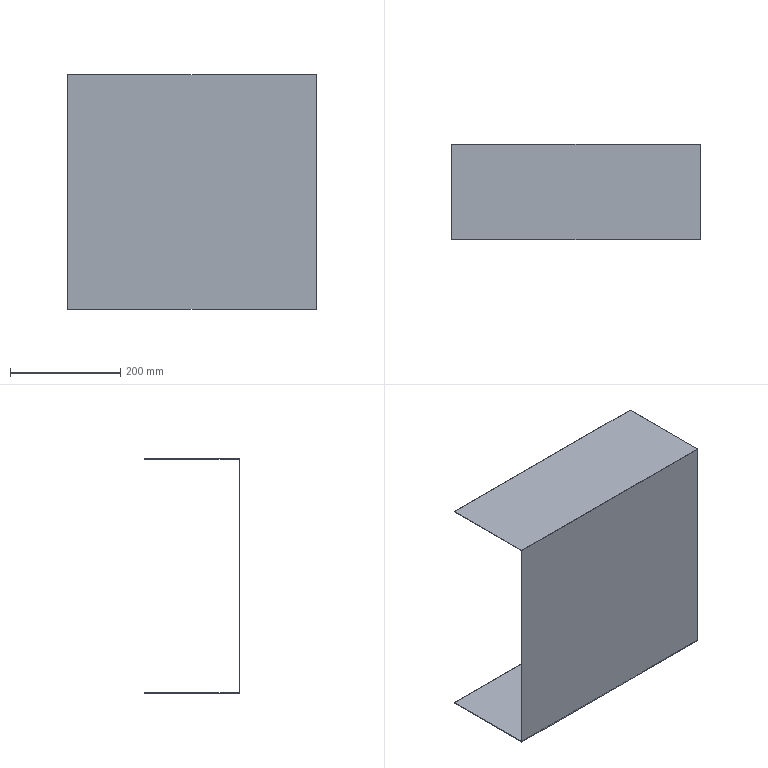Part | STEP file | Chassis side seal plate B_RR | 1 solid | 10 faces | box 450 x 173 x 425 mm | volume 346050 mm3 | plane 10
STEP:
#1=CARTESIAN_POINT('',(0.,0.,0.));
#2=DIRECTION('',(0.,0.,1.));
#3=DIRECTION('',(1.,0.,0.));
#4=AXIS2_PLACEMENT_3D('',#1,#2,#3);
#5=CARTESIAN_POINT('',(225.,0.,212.5));
#6=VERTEX_POINT('',#5);
#7=CARTESIAN_POINT('',(225.,0.,-212.5));
#8=VERTEX_POINT('',#7);
#9=CARTESIAN_POINT('',(225.,0.,0.));
#10=DIRECTION('',(0.,0.,-1.));
#11=VECTOR('',#10,1.);
#12=LINE('',#9,#11);
#13=CARTESIAN_POINT('',(0.,0.,0.));
#14=DIRECTION('',(0.,1.,0.));
#15=DIRECTION('',(0.,0.,1.));
#16=AXIS2_PLACEMENT_3D('',#13,#14,#15);
#17=PLANE('',#16);
#18=CARTESIAN_POINT('',(0.,225.));
#19=DIRECTION('',(-1.,0.));
#20=VECTOR('',#19,1.);
#21=LINE('',#18,#20);
#22=(GEOMETRIC_REPRESENTATION_CONTEXT(2)PARAMETRIC_REPRESENTATION_CONTEXT()REPRESENTATION_CONTEXT('',''));
#23=DEFINITIONAL_REPRESENTATION('',(#21),#22);
#24=PCURVE('',#17,#23);
#25=CARTESIAN_POINT('',(225.,0.,212.5));
#26=DIRECTION('',(1.,0.,0.));
#27=DIRECTION('',(0.,0.,-1.));
#28=AXIS2_PLACEMENT_3D('',#25,#26,#27);
#29=PLANE('',#28);
#30=CARTESIAN_POINT('',(212.5,0.));
#31=DIRECTION('',(1.,0.));
#32=VECTOR('',#31,1.);
#33=LINE('',#30,#32);
#34=(GEOMETRIC_REPRESENTATION_CONTEXT(2)PARAMETRIC_REPRESENTATION_CONTEXT()REPRESENTATION_CONTEXT('',''));
#35=DEFINITIONAL_REPRESENTATION('',(#33),#34);
#36=PCURVE('',#29,#35);
#37=SURFACE_CURVE('',#12,(#24,#36),.PCURVE_S1.);
#38=EDGE_CURVE('',#6,#8,#37,.T.);
#39=ORIENTED_EDGE('',*,*,#38,.F.);
#40=CARTESIAN_POINT('',(-225.,0.,212.5));
#41=VERTEX_POINT('',#40);
#42=CARTESIAN_POINT('',(0.,0.,212.5));
#43=DIRECTION('',(1.,0.,0.));
#44=VECTOR('',#43,1.);
#45=LINE('',#42,#44);
#46=CARTESIAN_POINT('',(212.5,0.));
#47=DIRECTION('',(0.,1.));
#48=VECTOR('',#47,1.);
#49=LINE('',#46,#48);
#50=(GEOMETRIC_REPRESENTATION_CONTEXT(2)PARAMETRIC_REPRESENTATION_CONTEXT()REPRESENTATION_CONTEXT('',''));
#51=DEFINITIONAL_REPRESENTATION('',(#49),#50);
#52=PCURVE('',#17,#51);
#53=CARTESIAN_POINT('',(-225.,0.,212.5));
#54=DIRECTION('',(0.,0.,1.));
#55=DIRECTION('',(1.,0.,0.));
#56=AXIS2_PLACEMENT_3D('',#53,#54,#55);
#57=PLANE('',#56);
#58=CARTESIAN_POINT('',(225.,0.));
#59=DIRECTION('',(1.,0.));
#60=VECTOR('',#59,1.);
#61=LINE('',#58,#60);
#62=(GEOMETRIC_REPRESENTATION_CONTEXT(2)PARAMETRIC_REPRESENTATION_CONTEXT()REPRESENTATION_CONTEXT('',''));
#63=DEFINITIONAL_REPRESENTATION('',(#61),#62);
#64=PCURVE('',#57,#63);
#65=SURFACE_CURVE('',#45,(#52,#64),.PCURVE_S1.);
#66=EDGE_CURVE('',#41,#6,#65,.T.);
#67=ORIENTED_EDGE('',*,*,#66,.F.);
#68=CARTESIAN_POINT('',(-225.,0.,-212.5));
#69=VERTEX_POINT('',#68);
#70=CARTESIAN_POINT('',(-225.,0.,0.));
#71=DIRECTION('',(0.,0.,1.));
#72=VECTOR('',#71,1.);
#73=LINE('',#70,#72);
#74=CARTESIAN_POINT('',(0.,-225.));
#75=DIRECTION('',(1.,0.));
#76=VECTOR('',#75,1.);
#77=LINE('',#74,#76);
#78=(GEOMETRIC_REPRESENTATION_CONTEXT(2)PARAMETRIC_REPRESENTATION_CONTEXT()REPRESENTATION_CONTEXT('',''));
#79=DEFINITIONAL_REPRESENTATION('',(#77),#78);
#80=PCURVE('',#17,#79);
#81=CARTESIAN_POINT('',(-225.,0.,-212.5));
#82=DIRECTION('',(-1.,0.,0.));
#83=DIRECTION('',(0.,0.,1.));
#84=AXIS2_PLACEMENT_3D('',#81,#82,#83);
#85=PLANE('',#84);
#86=CARTESIAN_POINT('',(212.5,0.));
#87=DIRECTION('',(1.,0.));
#88=VECTOR('',#87,1.);
#89=LINE('',#86,#88);
#90=(GEOMETRIC_REPRESENTATION_CONTEXT(2)PARAMETRIC_REPRESENTATION_CONTEXT()REPRESENTATION_CONTEXT('',''));
#91=DEFINITIONAL_REPRESENTATION('',(#89),#90);
#92=PCURVE('',#85,#91);
#93=SURFACE_CURVE('',#73,(#80,#92),.PCURVE_S1.);
#94=EDGE_CURVE('',#69,#41,#93,.T.);
#95=ORIENTED_EDGE('',*,*,#94,.F.);
#96=CARTESIAN_POINT('',(0.,0.,-212.5));
#97=DIRECTION('',(-1.,0.,0.));
#98=VECTOR('',#97,1.);
#99=LINE('',#96,#98);
#100=CARTESIAN_POINT('',(-212.5,0.));
#101=DIRECTION('',(0.,-1.));
#102=VECTOR('',#101,1.);
#103=LINE('',#100,#102);
#104=(GEOMETRIC_REPRESENTATION_CONTEXT(2)PARAMETRIC_REPRESENTATION_CONTEXT()REPRESENTATION_CONTEXT('',''));
#105=DEFINITIONAL_REPRESENTATION('',(#103),#104);
#106=PCURVE('',#17,#105);
#107=CARTESIAN_POINT('',(225.,0.,-212.5));
#108=DIRECTION('',(0.,0.,-1.));
#109=DIRECTION('',(-1.,0.,0.));
#110=AXIS2_PLACEMENT_3D('',#107,#108,#109);
#111=PLANE('',#110);
#112=CARTESIAN_POINT('',(225.,0.));
#113=DIRECTION('',(1.,0.));
#114=VECTOR('',#113,1.);
#115=LINE('',#112,#114);
#116=(GEOMETRIC_REPRESENTATION_CONTEXT(2)PARAMETRIC_REPRESENTATION_CONTEXT()REPRESENTATION_CONTEXT('',''));
#117=DEFINITIONAL_REPRESENTATION('',(#115),#116);
#118=PCURVE('',#111,#117);
#119=SURFACE_CURVE('',#99,(#106,#118),.PCURVE_S1.);
#120=EDGE_CURVE('',#8,#69,#119,.T.);
#121=ORIENTED_EDGE('',*,*,#120,.F.);
#122=EDGE_LOOP('',(#39,#67,#95,#121));
#123=FACE_BOUND('',#122,.T.);
#124=ADVANCED_FACE('',(#123),#17,.F.);
#125=CARTESIAN_POINT('',(225.,173.,-212.5));
#126=VERTEX_POINT('',#125);
#127=CARTESIAN_POINT('',(225.,0.,-212.5));
#128=DIRECTION('',(0.,-1.,0.));
#129=VECTOR('',#128,1.);
#130=LINE('',#127,#129);
#131=CARTESIAN_POINT('',(0.,0.));
#132=DIRECTION('',(0.,-1.));
#133=VECTOR('',#132,1.);
#134=LINE('',#131,#133);
#135=(GEOMETRIC_REPRESENTATION_CONTEXT(2)PARAMETRIC_REPRESENTATION_CONTEXT()REPRESENTATION_CONTEXT('',''));
#136=DEFINITIONAL_REPRESENTATION('',(#134),#135);
#137=PCURVE('',#111,#136);
#138=CARTESIAN_POINT('',(425.,0.));
#139=DIRECTION('',(0.,-1.));
#140=VECTOR('',#139,1.);
#141=LINE('',#138,#140);
#142=(GEOMETRIC_REPRESENTATION_CONTEXT(2)PARAMETRIC_REPRESENTATION_CONTEXT()REPRESENTATION_CONTEXT('',''));
#143=DEFINITIONAL_REPRESENTATION('',(#141),#142);
#144=PCURVE('',#29,#143);
#145=SURFACE_CURVE('',#130,(#137,#144),.PCURVE_S1.);
#146=EDGE_CURVE('',#126,#8,#145,.T.);
#147=ORIENTED_EDGE('',*,*,#146,.T.);
#148=ORIENTED_EDGE('',*,*,#120,.T.);
#149=CARTESIAN_POINT('',(-225.,173.,-212.5));
#150=VERTEX_POINT('',#149);
#151=CARTESIAN_POINT('',(-225.,0.,-212.5));
#152=DIRECTION('',(0.,1.,0.));
#153=VECTOR('',#152,1.);
#154=LINE('',#151,#153);
#155=CARTESIAN_POINT('',(450.,0.));
#156=DIRECTION('',(0.,1.));
#157=VECTOR('',#156,1.);
#158=LINE('',#155,#157);
#159=(GEOMETRIC_REPRESENTATION_CONTEXT(2)PARAMETRIC_REPRESENTATION_CONTEXT()REPRESENTATION_CONTEXT('',''));
#160=DEFINITIONAL_REPRESENTATION('',(#158),#159);
#161=PCURVE('',#111,#160);
#162=CARTESIAN_POINT('',(0.,0.));
#163=DIRECTION('',(0.,1.));
#164=VECTOR('',#163,1.);
#165=LINE('',#162,#164);
#166=(GEOMETRIC_REPRESENTATION_CONTEXT(2)PARAMETRIC_REPRESENTATION_CONTEXT()REPRESENTATION_CONTEXT('',''));
#167=DEFINITIONAL_REPRESENTATION('',(#165),#166);
#168=PCURVE('',#85,#167);
#169=SURFACE_CURVE('',#154,(#161,#168),.PCURVE_S1.);
#170=EDGE_CURVE('',#69,#150,#169,.T.);
#171=ORIENTED_EDGE('',*,*,#170,.T.);
#172=CARTESIAN_POINT('',(225.,173.,-212.5));
#173=DIRECTION('',(1.,0.,0.));
#174=VECTOR('',#173,1.);
#175=LINE('',#172,#174);
#176=CARTESIAN_POINT('',(0.,173.));
#177=DIRECTION('',(-1.,0.));
#178=VECTOR('',#177,1.);
#179=LINE('',#176,#178);
#180=(GEOMETRIC_REPRESENTATION_CONTEXT(2)PARAMETRIC_REPRESENTATION_CONTEXT()REPRESENTATION_CONTEXT('',''));
#181=DEFINITIONAL_REPRESENTATION('',(#179),#180);
#182=PCURVE('',#111,#181);
#183=CARTESIAN_POINT('',(0.,173.,0.));
#184=DIRECTION('',(0.,1.,0.));
#185=DIRECTION('',(0.,0.,1.));
#186=AXIS2_PLACEMENT_3D('',#183,#184,#185);
#187=PLANE('',#186);
#188=CARTESIAN_POINT('',(-212.5,225.));
#189=DIRECTION('',(0.,1.));
#190=VECTOR('',#189,1.);
#191=LINE('',#188,#190);
#192=(GEOMETRIC_REPRESENTATION_CONTEXT(2)PARAMETRIC_REPRESENTATION_CONTEXT()REPRESENTATION_CONTEXT('',''));
#193=DEFINITIONAL_REPRESENTATION('',(#191),#192);
#194=PCURVE('',#187,#193);
#195=SURFACE_CURVE('',#175,(#182,#194),.PCURVE_S1.);
#196=EDGE_CURVE('',#150,#126,#195,.T.);
#197=ORIENTED_EDGE('',*,*,#196,.T.);
#198=EDGE_LOOP('',(#147,#148,#171,#197));
#199=FACE_BOUND('',#198,.T.);
#200=ADVANCED_FACE('',(#199),#111,.T.);
#201=CARTESIAN_POINT('',(225.,173.,-211.5));
#202=VERTEX_POINT('',#201);
#203=CARTESIAN_POINT('',(225.,1.,-211.5));
#204=VERTEX_POINT('',#203);
#205=CARTESIAN_POINT('',(225.,0.,-211.5));
#206=DIRECTION('',(0.,-1.,0.));
#207=VECTOR('',#206,1.);
#208=LINE('',#205,#207);
#209=CARTESIAN_POINT('',(424.,0.));
#210=DIRECTION('',(0.,-1.));
#211=VECTOR('',#210,1.);
#212=LINE('',#209,#211);
#213=(GEOMETRIC_REPRESENTATION_CONTEXT(2)PARAMETRIC_REPRESENTATION_CONTEXT()REPRESENTATION_CONTEXT('',''));
#214=DEFINITIONAL_REPRESENTATION('',(#212),#213);
#215=PCURVE('',#29,#214);
#216=CARTESIAN_POINT('',(225.,0.,-211.5));
#217=DIRECTION('',(0.,0.,-1.));
#218=DIRECTION('',(-1.,0.,0.));
#219=AXIS2_PLACEMENT_3D('',#216,#217,#218);
#220=PLANE('',#219);
#221=CARTESIAN_POINT('',(0.,0.));
#222=DIRECTION('',(0.,-1.));
#223=VECTOR('',#222,1.);
#224=LINE('',#221,#223);
#225=(GEOMETRIC_REPRESENTATION_CONTEXT(2)PARAMETRIC_REPRESENTATION_CONTEXT()REPRESENTATION_CONTEXT('',''));
#226=DEFINITIONAL_REPRESENTATION('',(#224),#225);
#227=PCURVE('',#220,#226);
#228=SURFACE_CURVE('',#208,(#215,#227),.PCURVE_S1.);
#229=EDGE_CURVE('',#202,#204,#228,.T.);
#230=ORIENTED_EDGE('',*,*,#229,.T.);
#231=CARTESIAN_POINT('',(225.,1.,211.5));
#232=VERTEX_POINT('',#231);
#233=CARTESIAN_POINT('',(225.,1.,212.5));
#234=DIRECTION('',(0.,0.,1.));
#235=VECTOR('',#234,1.);
#236=LINE('',#233,#235);
#237=CARTESIAN_POINT('',(0.,1.));
#238=DIRECTION('',(-1.,0.));
#239=VECTOR('',#238,1.);
#240=LINE('',#237,#239);
#241=(GEOMETRIC_REPRESENTATION_CONTEXT(2)PARAMETRIC_REPRESENTATION_CONTEXT()REPRESENTATION_CONTEXT('',''));
#242=DEFINITIONAL_REPRESENTATION('',(#240),#241);
#243=PCURVE('',#29,#242);
#244=CARTESIAN_POINT('',(0.,1.,0.));
#245=DIRECTION('',(0.,1.,0.));
#246=DIRECTION('',(0.,0.,1.));
#247=AXIS2_PLACEMENT_3D('',#244,#245,#246);
#248=PLANE('',#247);
#249=CARTESIAN_POINT('',(212.5,225.));
#250=DIRECTION('',(1.,0.));
#251=VECTOR('',#250,1.);
#252=LINE('',#249,#251);
#253=(GEOMETRIC_REPRESENTATION_CONTEXT(2)PARAMETRIC_REPRESENTATION_CONTEXT()REPRESENTATION_CONTEXT('',''));
#254=DEFINITIONAL_REPRESENTATION('',(#252),#253);
#255=PCURVE('',#248,#254);
#256=SURFACE_CURVE('',#236,(#243,#255),.PCURVE_S1.);
#257=EDGE_CURVE('',#204,#232,#256,.T.);
#258=ORIENTED_EDGE('',*,*,#257,.T.);
#259=CARTESIAN_POINT('',(225.,173.,211.5));
#260=VERTEX_POINT('',#259);
#261=CARTESIAN_POINT('',(225.,0.,211.5));
#262=DIRECTION('',(0.,1.,0.));
#263=VECTOR('',#262,1.);
#264=LINE('',#261,#263);
#265=CARTESIAN_POINT('',(1.,0.));
#266=DIRECTION('',(0.,1.));
#267=VECTOR('',#266,1.);
#268=LINE('',#265,#267);
#269=(GEOMETRIC_REPRESENTATION_CONTEXT(2)PARAMETRIC_REPRESENTATION_CONTEXT()REPRESENTATION_CONTEXT('',''));
#270=DEFINITIONAL_REPRESENTATION('',(#268),#269);
#271=PCURVE('',#29,#270);
#272=CARTESIAN_POINT('',(-225.,0.,211.5));
#273=DIRECTION('',(0.,0.,1.));
#274=DIRECTION('',(1.,0.,0.));
#275=AXIS2_PLACEMENT_3D('',#272,#273,#274);
#276=PLANE('',#275);
#277=CARTESIAN_POINT('',(450.,0.));
#278=DIRECTION('',(0.,1.));
#279=VECTOR('',#278,1.);
#280=LINE('',#277,#279);
#281=(GEOMETRIC_REPRESENTATION_CONTEXT(2)PARAMETRIC_REPRESENTATION_CONTEXT()REPRESENTATION_CONTEXT('',''));
#282=DEFINITIONAL_REPRESENTATION('',(#280),#281);
#283=PCURVE('',#276,#282);
#284=SURFACE_CURVE('',#264,(#271,#283),.PCURVE_S1.);
#285=EDGE_CURVE('',#232,#260,#284,.T.);
#286=ORIENTED_EDGE('',*,*,#285,.T.);
#287=CARTESIAN_POINT('',(225.,173.,212.5));
#288=VERTEX_POINT('',#287);
#289=CARTESIAN_POINT('',(225.,173.,0.));
#290=DIRECTION('',(0.,0.,-1.));
#291=VECTOR('',#290,1.);
#292=LINE('',#289,#291);
#293=CARTESIAN_POINT('',(212.5,173.));
#294=DIRECTION('',(1.,0.));
#295=VECTOR('',#294,1.);
#296=LINE('',#293,#295);
#297=(GEOMETRIC_REPRESENTATION_CONTEXT(2)PARAMETRIC_REPRESENTATION_CONTEXT()REPRESENTATION_CONTEXT('',''));
#298=DEFINITIONAL_REPRESENTATION('',(#296),#297);
#299=PCURVE('',#29,#298);
#300=CARTESIAN_POINT('',(0.,173.,0.));
#301=DIRECTION('',(0.,1.,0.));
#302=DIRECTION('',(0.,0.,1.));
#303=AXIS2_PLACEMENT_3D('',#300,#301,#302);
#304=PLANE('',#303);
#305=CARTESIAN_POINT('',(0.,225.));
#306=DIRECTION('',(-1.,0.));
#307=VECTOR('',#306,1.);
#308=LINE('',#305,#307);
#309=(GEOMETRIC_REPRESENTATION_CONTEXT(2)PARAMETRIC_REPRESENTATION_CONTEXT()REPRESENTATION_CONTEXT('',''));
#310=DEFINITIONAL_REPRESENTATION('',(#308),#309);
#311=PCURVE('',#304,#310);
#312=SURFACE_CURVE('',#292,(#299,#311),.PCURVE_S1.);
#313=EDGE_CURVE('',#288,#260,#312,.T.);
#314=ORIENTED_EDGE('',*,*,#313,.F.);
#315=CARTESIAN_POINT('',(225.,0.,212.5));
#316=DIRECTION('',(0.,-1.,0.));
#317=VECTOR('',#316,1.);
#318=LINE('',#315,#317);
#319=CARTESIAN_POINT('',(0.,0.));
#320=DIRECTION('',(0.,-1.));
#321=VECTOR('',#320,1.);
#322=LINE('',#319,#321);
#323=(GEOMETRIC_REPRESENTATION_CONTEXT(2)PARAMETRIC_REPRESENTATION_CONTEXT()REPRESENTATION_CONTEXT('',''));
#324=DEFINITIONAL_REPRESENTATION('',(#322),#323);
#325=PCURVE('',#29,#324);
#326=CARTESIAN_POINT('',(450.,0.));
#327=DIRECTION('',(0.,-1.));
#328=VECTOR('',#327,1.);
#329=LINE('',#326,#328);
#330=(GEOMETRIC_REPRESENTATION_CONTEXT(2)PARAMETRIC_REPRESENTATION_CONTEXT()REPRESENTATION_CONTEXT('',''));
#331=DEFINITIONAL_REPRESENTATION('',(#329),#330);
#332=PCURVE('',#57,#331);
#333=SURFACE_CURVE('',#318,(#325,#332),.PCURVE_S1.);
#334=EDGE_CURVE('',#288,#6,#333,.T.);
#335=ORIENTED_EDGE('',*,*,#334,.T.);
#336=ORIENTED_EDGE('',*,*,#38,.T.);
#337=ORIENTED_EDGE('',*,*,#146,.F.);
#338=CARTESIAN_POINT('',(225.,173.,212.5));
#339=DIRECTION('',(0.,0.,1.));
#340=VECTOR('',#339,1.);
#341=LINE('',#338,#340);
#342=CARTESIAN_POINT('',(0.,173.));
#343=DIRECTION('',(-1.,0.));
#344=VECTOR('',#343,1.);
#345=LINE('',#342,#344);
#346=(GEOMETRIC_REPRESENTATION_CONTEXT(2)PARAMETRIC_REPRESENTATION_CONTEXT()REPRESENTATION_CONTEXT('',''));
#347=DEFINITIONAL_REPRESENTATION('',(#345),#346);
#348=PCURVE('',#29,#347);
#349=CARTESIAN_POINT('',(212.5,225.));
#350=DIRECTION('',(1.,0.));
#351=VECTOR('',#350,1.);
#352=LINE('',#349,#351);
#353=(GEOMETRIC_REPRESENTATION_CONTEXT(2)PARAMETRIC_REPRESENTATION_CONTEXT()REPRESENTATION_CONTEXT('',''));
#354=DEFINITIONAL_REPRESENTATION('',(#352),#353);
#355=PCURVE('',#187,#354);
#356=SURFACE_CURVE('',#341,(#348,#355),.PCURVE_S1.);
#357=EDGE_CURVE('',#126,#202,#356,.T.);
#358=ORIENTED_EDGE('',*,*,#357,.T.);
#359=EDGE_LOOP('',(#230,#258,#286,#314,#335,#336,#337,#358));
#360=FACE_BOUND('',#359,.T.);
#361=ADVANCED_FACE('',(#360),#29,.T.);
#362=CARTESIAN_POINT('',(-225.,173.,212.5));
#363=VERTEX_POINT('',#362);
#364=CARTESIAN_POINT('',(-225.,0.,212.5));
#365=DIRECTION('',(0.,-1.,0.));
#366=VECTOR('',#365,1.);
#367=LINE('',#364,#366);
#368=CARTESIAN_POINT('',(0.,0.));
#369=DIRECTION('',(0.,-1.));
#370=VECTOR('',#369,1.);
#371=LINE('',#368,#370);
#372=(GEOMETRIC_REPRESENTATION_CONTEXT(2)PARAMETRIC_REPRESENTATION_CONTEXT()REPRESENTATION_CONTEXT('',''));
#373=DEFINITIONAL_REPRESENTATION('',(#371),#372);
#374=PCURVE('',#57,#373);
#375=CARTESIAN_POINT('',(425.,0.));
#376=DIRECTION('',(0.,-1.));
#377=VECTOR('',#376,1.);
#378=LINE('',#375,#377);
#379=(GEOMETRIC_REPRESENTATION_CONTEXT(2)PARAMETRIC_REPRESENTATION_CONTEXT()REPRESENTATION_CONTEXT('',''));
#380=DEFINITIONAL_REPRESENTATION('',(#378),#379);
#381=PCURVE('',#85,#380);
#382=SURFACE_CURVE('',#367,(#374,#381),.PCURVE_S1.);
#383=EDGE_CURVE('',#363,#41,#382,.T.);
#384=ORIENTED_EDGE('',*,*,#383,.T.);
#385=ORIENTED_EDGE('',*,*,#66,.T.);
#386=ORIENTED_EDGE('',*,*,#334,.F.);
#387=CARTESIAN_POINT('',(-225.,173.,212.5));
#388=DIRECTION('',(-1.,0.,0.));
#389=VECTOR('',#388,1.);
#390=LINE('',#387,#389);
#391=CARTESIAN_POINT('',(0.,173.));
#392=DIRECTION('',(-1.,0.));
#393=VECTOR('',#392,1.);
#394=LINE('',#391,#393);
#395=(GEOMETRIC_REPRESENTATION_CONTEXT(2)PARAMETRIC_REPRESENTATION_CONTEXT()REPRESENTATION_CONTEXT('',''));
#396=DEFINITIONAL_REPRESENTATION('',(#394),#395);
#397=PCURVE('',#57,#396);
#398=CARTESIAN_POINT('',(212.5,-225.));
#399=DIRECTION('',(0.,-1.));
#400=VECTOR('',#399,1.);
#401=LINE('',#398,#400);
#402=(GEOMETRIC_REPRESENTATION_CONTEXT(2)PARAMETRIC_REPRESENTATION_CONTEXT()REPRESENTATION_CONTEXT('',''));
#403=DEFINITIONAL_REPRESENTATION('',(#401),#402);
#404=PCURVE('',#304,#403);
#405=SURFACE_CURVE('',#390,(#397,#404),.PCURVE_S1.);
#406=EDGE_CURVE('',#288,#363,#405,.T.);
#407=ORIENTED_EDGE('',*,*,#406,.T.);
#408=EDGE_LOOP('',(#384,#385,#386,#407));
#409=FACE_BOUND('',#408,.T.);
#410=ADVANCED_FACE('',(#409),#57,.T.);
#411=CARTESIAN_POINT('',(-225.,173.,211.5));
#412=VERTEX_POINT('',#411);
#413=CARTESIAN_POINT('',(-225.,1.,211.5));
#414=VERTEX_POINT('',#413);
#415=CARTESIAN_POINT('',(-225.,0.,211.5));
#416=DIRECTION('',(0.,-1.,0.));
#417=VECTOR('',#416,1.);
#418=LINE('',#415,#417);
#419=CARTESIAN_POINT('',(424.,0.));
#420=DIRECTION('',(0.,-1.));
#421=VECTOR('',#420,1.);
#422=LINE('',#419,#421);
#423=(GEOMETRIC_REPRESENTATION_CONTEXT(2)PARAMETRIC_REPRESENTATION_CONTEXT()REPRESENTATION_CONTEXT('',''));
#424=DEFINITIONAL_REPRESENTATION('',(#422),#423);
#425=PCURVE('',#85,#424);
#426=CARTESIAN_POINT('',(0.,0.));
#427=DIRECTION('',(0.,-1.));
#428=VECTOR('',#427,1.);
#429=LINE('',#426,#428);
#430=(GEOMETRIC_REPRESENTATION_CONTEXT(2)PARAMETRIC_REPRESENTATION_CONTEXT()REPRESENTATION_CONTEXT('',''));
#431=DEFINITIONAL_REPRESENTATION('',(#429),#430);
#432=PCURVE('',#276,#431);
#433=SURFACE_CURVE('',#418,(#425,#432),.PCURVE_S1.);
#434=EDGE_CURVE('',#412,#414,#433,.T.);
#435=ORIENTED_EDGE('',*,*,#434,.T.);
#436=CARTESIAN_POINT('',(-225.,1.,-211.5));
#437=VERTEX_POINT('',#436);
#438=CARTESIAN_POINT('',(-225.,1.,-212.5));
#439=DIRECTION('',(0.,0.,-1.));
#440=VECTOR('',#439,1.);
#441=LINE('',#438,#440);
#442=CARTESIAN_POINT('',(0.,1.));
#443=DIRECTION('',(-1.,0.));
#444=VECTOR('',#443,1.);
#445=LINE('',#442,#444);
#446=(GEOMETRIC_REPRESENTATION_CONTEXT(2)PARAMETRIC_REPRESENTATION_CONTEXT()REPRESENTATION_CONTEXT('',''));
#447=DEFINITIONAL_REPRESENTATION('',(#445),#446);
#448=PCURVE('',#85,#447);
#449=CARTESIAN_POINT('',(-212.5,-225.));
#450=DIRECTION('',(-1.,0.));
#451=VECTOR('',#450,1.);
#452=LINE('',#449,#451);
#453=(GEOMETRIC_REPRESENTATION_CONTEXT(2)PARAMETRIC_REPRESENTATION_CONTEXT()REPRESENTATION_CONTEXT('',''));
#454=DEFINITIONAL_REPRESENTATION('',(#452),#453);
#455=PCURVE('',#248,#454);
#456=SURFACE_CURVE('',#441,(#448,#455),.PCURVE_S1.);
#457=EDGE_CURVE('',#414,#437,#456,.T.);
#458=ORIENTED_EDGE('',*,*,#457,.T.);
#459=CARTESIAN_POINT('',(-225.,173.,-211.5));
#460=VERTEX_POINT('',#459);
#461=CARTESIAN_POINT('',(-225.,0.,-211.5));
#462=DIRECTION('',(0.,1.,0.));
#463=VECTOR('',#462,1.);
#464=LINE('',#461,#463);
#465=CARTESIAN_POINT('',(1.,0.));
#466=DIRECTION('',(0.,1.));
#467=VECTOR('',#466,1.);
#468=LINE('',#465,#467);
#469=(GEOMETRIC_REPRESENTATION_CONTEXT(2)PARAMETRIC_REPRESENTATION_CONTEXT()REPRESENTATION_CONTEXT('',''));
#470=DEFINITIONAL_REPRESENTATION('',(#468),#469);
#471=PCURVE('',#85,#470);
#472=CARTESIAN_POINT('',(450.,0.));
#473=DIRECTION('',(0.,1.));
#474=VECTOR('',#473,1.);
#475=LINE('',#472,#474);
#476=(GEOMETRIC_REPRESENTATION_CONTEXT(2)PARAMETRIC_REPRESENTATION_CONTEXT()REPRESENTATION_CONTEXT('',''));
#477=DEFINITIONAL_REPRESENTATION('',(#475),#476);
#478=PCURVE('',#220,#477);
#479=SURFACE_CURVE('',#464,(#471,#478),.PCURVE_S1.);
#480=EDGE_CURVE('',#437,#460,#479,.T.);
#481=ORIENTED_EDGE('',*,*,#480,.T.);
#482=CARTESIAN_POINT('',(-225.,173.,-212.5));
#483=DIRECTION('',(0.,0.,-1.));
#484=VECTOR('',#483,1.);
#485=LINE('',#482,#484);
#486=CARTESIAN_POINT('',(0.,173.));
#487=DIRECTION('',(-1.,0.));
#488=VECTOR('',#487,1.);
#489=LINE('',#486,#488);
#490=(GEOMETRIC_REPRESENTATION_CONTEXT(2)PARAMETRIC_REPRESENTATION_CONTEXT()REPRESENTATION_CONTEXT('',''));
#491=DEFINITIONAL_REPRESENTATION('',(#489),#490);
#492=PCURVE('',#85,#491);
#493=CARTESIAN_POINT('',(-212.5,-225.));
#494=DIRECTION('',(-1.,0.));
#495=VECTOR('',#494,1.);
#496=LINE('',#493,#495);
#497=(GEOMETRIC_REPRESENTATION_CONTEXT(2)PARAMETRIC_REPRESENTATION_CONTEXT()REPRESENTATION_CONTEXT('',''));
#498=DEFINITIONAL_REPRESENTATION('',(#496),#497);
#499=PCURVE('',#187,#498);
#500=SURFACE_CURVE('',#485,(#492,#499),.PCURVE_S1.);
#501=EDGE_CURVE('',#460,#150,#500,.T.);
#502=ORIENTED_EDGE('',*,*,#501,.T.);
#503=ORIENTED_EDGE('',*,*,#170,.F.);
#504=ORIENTED_EDGE('',*,*,#94,.T.);
#505=ORIENTED_EDGE('',*,*,#383,.F.);
#506=CARTESIAN_POINT('',(-225.,173.,-212.5));
#507=DIRECTION('',(0.,0.,-1.));
#508=VECTOR('',#507,1.);
#509=LINE('',#506,#508);
#510=CARTESIAN_POINT('',(0.,173.));
#511=DIRECTION('',(-1.,0.));
#512=VECTOR('',#511,1.);
#513=LINE('',#510,#512);
#514=(GEOMETRIC_REPRESENTATION_CONTEXT(2)PARAMETRIC_REPRESENTATION_CONTEXT()REPRESENTATION_CONTEXT('',''));
#515=DEFINITIONAL_REPRESENTATION('',(#513),#514);
#516=PCURVE('',#85,#515);
#517=CARTESIAN_POINT('',(-212.5,-225.));
#518=DIRECTION('',(-1.,0.));
#519=VECTOR('',#518,1.);
#520=LINE('',#517,#519);
#521=(GEOMETRIC_REPRESENTATION_CONTEXT(2)PARAMETRIC_REPRESENTATION_CONTEXT()REPRESENTATION_CONTEXT('',''));
#522=DEFINITIONAL_REPRESENTATION('',(#520),#521);
#523=PCURVE('',#304,#522);
#524=SURFACE_CURVE('',#509,(#516,#523),.PCURVE_S1.);
#525=EDGE_CURVE('',#363,#412,#524,.T.);
#526=ORIENTED_EDGE('',*,*,#525,.T.);
#527=EDGE_LOOP('',(#435,#458,#481,#502,#503,#504,#505,#526));
#528=FACE_BOUND('',#527,.T.);
#529=ADVANCED_FACE('',(#528),#85,.T.);
#530=ORIENTED_EDGE('',*,*,#501,.F.);
#531=CARTESIAN_POINT('',(0.,173.,-211.5));
#532=DIRECTION('',(1.,0.,0.));
#533=VECTOR('',#532,1.);
#534=LINE('',#531,#533);
#535=CARTESIAN_POINT('',(-211.5,0.));
#536=DIRECTION('',(0.,1.));
#537=VECTOR('',#536,1.);
#538=LINE('',#535,#537);
#539=(GEOMETRIC_REPRESENTATION_CONTEXT(2)PARAMETRIC_REPRESENTATION_CONTEXT()REPRESENTATION_CONTEXT('',''));
#540=DEFINITIONAL_REPRESENTATION('',(#538),#539);
#541=PCURVE('',#187,#540);
#542=CARTESIAN_POINT('',(225.,173.));
#543=DIRECTION('',(-1.,0.));
#544=VECTOR('',#543,1.);
#545=LINE('',#542,#544);
#546=(GEOMETRIC_REPRESENTATION_CONTEXT(2)PARAMETRIC_REPRESENTATION_CONTEXT()REPRESENTATION_CONTEXT('',''));
#547=DEFINITIONAL_REPRESENTATION('',(#545),#546);
#548=PCURVE('',#220,#547);
#549=SURFACE_CURVE('',#534,(#541,#548),.PCURVE_S1.);
#550=EDGE_CURVE('',#460,#202,#549,.T.);
#551=ORIENTED_EDGE('',*,*,#550,.T.);
#552=ORIENTED_EDGE('',*,*,#357,.F.);
#553=ORIENTED_EDGE('',*,*,#196,.F.);
#554=EDGE_LOOP('',(#530,#551,#552,#553));
#555=FACE_BOUND('',#554,.T.);
#556=ADVANCED_FACE('',(#555),#187,.T.);
#557=CARTESIAN_POINT('',(0.,1.,-211.5));
#558=DIRECTION('',(-1.,0.,0.));
#559=VECTOR('',#558,1.);
#560=LINE('',#557,#559);
#561=CARTESIAN_POINT('',(-211.5,0.));
#562=DIRECTION('',(0.,-1.));
#563=VECTOR('',#562,1.);
#564=LINE('',#561,#563);
#565=(GEOMETRIC_REPRESENTATION_CONTEXT(2)PARAMETRIC_REPRESENTATION_CONTEXT()REPRESENTATION_CONTEXT('',''));
#566=DEFINITIONAL_REPRESENTATION('',(#564),#565);
#567=PCURVE('',#248,#566);
#568=CARTESIAN_POINT('',(225.,1.));
#569=DIRECTION('',(1.,0.));
#570=VECTOR('',#569,1.);
#571=LINE('',#568,#570);
#572=(GEOMETRIC_REPRESENTATION_CONTEXT(2)PARAMETRIC_REPRESENTATION_CONTEXT()REPRESENTATION_CONTEXT('',''));
#573=DEFINITIONAL_REPRESENTATION('',(#571),#572);
#574=PCURVE('',#220,#573);
#575=SURFACE_CURVE('',#560,(#567,#574),.PCURVE_S1.);
#576=EDGE_CURVE('',#204,#437,#575,.T.);
#577=ORIENTED_EDGE('',*,*,#576,.T.);
#578=ORIENTED_EDGE('',*,*,#457,.F.);
#579=CARTESIAN_POINT('',(0.,1.,211.5));
#580=DIRECTION('',(1.,0.,0.));
#581=VECTOR('',#580,1.);
#582=LINE('',#579,#581);
#583=CARTESIAN_POINT('',(211.5,0.));
#584=DIRECTION('',(0.,1.));
#585=VECTOR('',#584,1.);
#586=LINE('',#583,#585);
#587=(GEOMETRIC_REPRESENTATION_CONTEXT(2)PARAMETRIC_REPRESENTATION_CONTEXT()REPRESENTATION_CONTEXT('',''));
#588=DEFINITIONAL_REPRESENTATION('',(#586),#587);
#589=PCURVE('',#248,#588);
#590=CARTESIAN_POINT('',(225.,1.));
#591=DIRECTION('',(1.,0.));
#592=VECTOR('',#591,1.);
#593=LINE('',#590,#592);
#594=(GEOMETRIC_REPRESENTATION_CONTEXT(2)PARAMETRIC_REPRESENTATION_CONTEXT()REPRESENTATION_CONTEXT('',''));
#595=DEFINITIONAL_REPRESENTATION('',(#593),#594);
#596=PCURVE('',#276,#595);
#597=SURFACE_CURVE('',#582,(#589,#596),.PCURVE_S1.);
#598=EDGE_CURVE('',#414,#232,#597,.T.);
#599=ORIENTED_EDGE('',*,*,#598,.T.);
#600=ORIENTED_EDGE('',*,*,#257,.F.);
#601=EDGE_LOOP('',(#577,#578,#599,#600));
#602=FACE_BOUND('',#601,.T.);
#603=ADVANCED_FACE('',(#602),#248,.T.);
#604=ORIENTED_EDGE('',*,*,#576,.F.);
#605=ORIENTED_EDGE('',*,*,#229,.F.);
#606=ORIENTED_EDGE('',*,*,#550,.F.);
#607=ORIENTED_EDGE('',*,*,#480,.F.);
#608=EDGE_LOOP('',(#604,#605,#606,#607));
#609=FACE_BOUND('',#608,.T.);
#610=ADVANCED_FACE('',(#609),#220,.F.);
#611=ORIENTED_EDGE('',*,*,#598,.F.);
#612=ORIENTED_EDGE('',*,*,#434,.F.);
#613=CARTESIAN_POINT('',(-225.,173.,211.5));
#614=DIRECTION('',(-1.,0.,0.));
#615=VECTOR('',#614,1.);
#616=LINE('',#613,#615);
#617=CARTESIAN_POINT('',(0.,173.));
#618=DIRECTION('',(-1.,0.));
#619=VECTOR('',#618,1.);
#620=LINE('',#617,#619);
#621=(GEOMETRIC_REPRESENTATION_CONTEXT(2)PARAMETRIC_REPRESENTATION_CONTEXT()REPRESENTATION_CONTEXT('',''));
#622=DEFINITIONAL_REPRESENTATION('',(#620),#621);
#623=PCURVE('',#276,#622);
#624=CARTESIAN_POINT('',(211.5,-225.));
#625=DIRECTION('',(0.,-1.));
#626=VECTOR('',#625,1.);
#627=LINE('',#624,#626);
#628=(GEOMETRIC_REPRESENTATION_CONTEXT(2)PARAMETRIC_REPRESENTATION_CONTEXT()REPRESENTATION_CONTEXT('',''));
#629=DEFINITIONAL_REPRESENTATION('',(#627),#628);
#630=PCURVE('',#304,#629);
#631=SURFACE_CURVE('',#616,(#623,#630),.PCURVE_S1.);
#632=EDGE_CURVE('',#260,#412,#631,.T.);
#633=ORIENTED_EDGE('',*,*,#632,.F.);
#634=ORIENTED_EDGE('',*,*,#285,.F.);
#635=EDGE_LOOP('',(#611,#612,#633,#634));
#636=FACE_BOUND('',#635,.T.);
#637=ADVANCED_FACE('',(#636),#276,.F.);
#638=ORIENTED_EDGE('',*,*,#313,.T.);
#639=ORIENTED_EDGE('',*,*,#632,.T.);
#640=ORIENTED_EDGE('',*,*,#525,.F.);
#641=ORIENTED_EDGE('',*,*,#406,.F.);
#642=EDGE_LOOP('',(#638,#639,#640,#641));
#643=FACE_BOUND('',#642,.T.);
#644=ADVANCED_FACE('',(#643),#304,.T.);
#645=CLOSED_SHELL('',(#124,#200,#361,#410,#529,#556,#603,#610,#637,#644));
#646=MANIFOLD_SOLID_BREP('',#645);
#647=(LENGTH_UNIT()NAMED_UNIT(*)SI_UNIT(.MILLI.,.METRE.));
#648=UNCERTAINTY_MEASURE_WITH_UNIT(LENGTH_MEASURE(0.0000001),#647,'','');
#649=(NAMED_UNIT(*)PLANE_ANGLE_UNIT()SI_UNIT($,.RADIAN.));
#650=(NAMED_UNIT(*)SI_UNIT($,.STERADIAN.)SOLID_ANGLE_UNIT());
#651=(GEOMETRIC_REPRESENTATION_CONTEXT(3)GLOBAL_UNCERTAINTY_ASSIGNED_CONTEXT((#648))GLOBAL_UNIT_ASSIGNED_CONTEXT((#647,#649,#650))REPRESENTATION_CONTEXT('',''));
#652=ADVANCED_BREP_SHAPE_REPRESENTATION('',(#4,#646),#651);